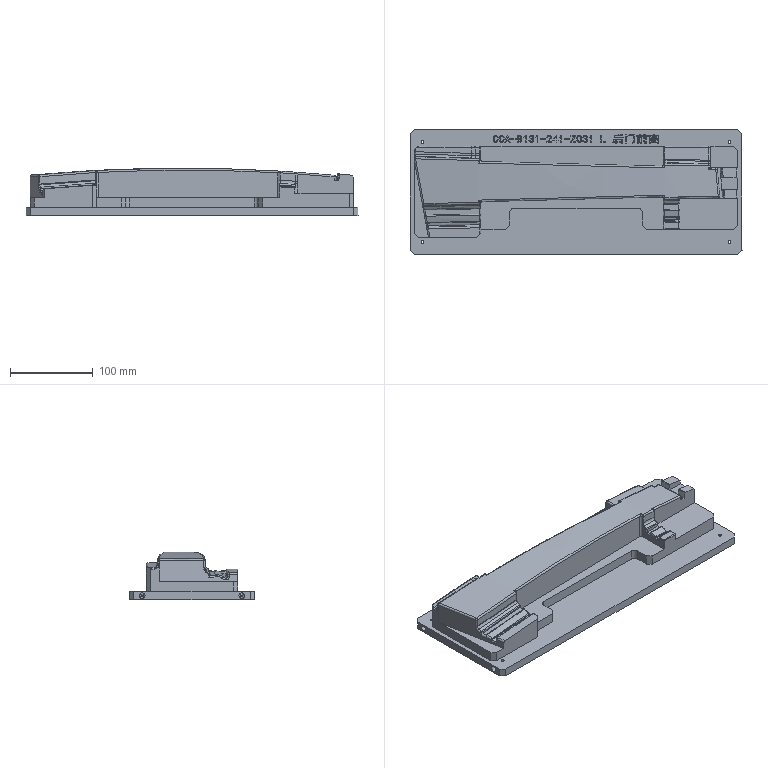NC program | NX | posted with a generic post | part box 400 x 150 x 57.494 mm
Lines 58 to 1056 of 7057:
(A4 , TOOL : D0.5)
N102 M6
N104 G54
N106 G17 G0 G90 X-99.468 Y63.115 S0 M3
N108 G43 Z20.002 H0
N110 Z10.302
N112 G94 G1 X-99.408 Y62.639 Z10.277 F250.
N114 X-99.26 Y62.087 Z10.247
N116 X-99.023 Y61.594 Z10.218
N118 X-98.688 Y61.174 Z10.19
N120 X-98.122 Y60.757 Z10.153
N122 X-98.359 Y60.946 Z10.137
N124 X-98.535 Y61.194 Z10.122
N126 X-98.911 Y61.942 Z10.078
N128 X-99.085 Y62.741 Z10.035
N130 X-99.146 Y63.516 Z9.994
N132 X-99.142 Y64.278 Z9.954
N134 X-99.139 Y64.316 Z9.952
N136 X-99.076 Y65.081
N138 X-98.905 Y65.905
N140 X-98.539 Y66.707
N142 X-98.173 Y67.122
N144 X-98.022 Y67.233
N146 G3 X-99.028 Y66.178 R2.627
N148 X-99.26 Y62.087 R6.192
N150 G1 X-99.023 Y61.594
N152 X-98.688 Y61.174
N154 X-98.268 Y60.845
N156 X-98.122 Y60.757
N158 G2 X-98.535 Y61.194 R2.143
N160 G1 X-98.911 Y61.942
N162 X-99.085 Y62.741
N164 X-99.146 Y63.516
N166 X-99.142 Y64.278
N168 X-99.139 Y64.316
N170 X-98.89 Y64.295
N172 X-98.828 Y65.045
N174 X-98.666 Y65.827
N176 G2 X-95.732 Y67.213 R2.025
N178 G1 X-95.663 Y67.169
N180 X-95.496 Y67.021
N182 X-95.329 Y67.207
N184 X-95.166 Y67.062
N186 X-95.083 Y67.017
N188 X-95.059 Y66.925
N190 X-94.818 Y66.478
N192 X-94.671 Y65.947
N194 X-94.646 Y65.644
N196 X-94.391
N198 X-94.568 Y66.329
N200 X-94.673 Y66.566
N202 X-94.957 Y66.932
N204 G3 X-95.329 Y67.207 R2.627
N206 G1 X-95.496 Y67.021
N208 X-95.333 Y66.875
N210 X-95.279 Y66.807
N212 X-95.051 Y66.384
N214 X-94.918 Y65.903
N216 X-94.876 Y65.394
N218 X-94.13
N220 X-94.222 Y66.097
N222 X-94.335 Y66.421
N224 X-94.456 Y66.696
N226 X-94.773 Y67.103
N228 G3 X-99.254 Y66.284 R2.877
N230 X-99.496 Y61.999 R6.441
N232 G1 X-99.236 Y61.461
N234 X-98.866 Y60.995
N236 X-98.414 Y60.642
N238 G3 X-95.389 Y60.515 R2.952
N240 G1 X-95.508 Y60.735
N242 G3 X-94.923 Y61.161 R2.702
N244 X-94.363 Y62.679 R2.769
N246 G1 X-94.628
N248 X-94.629 Y62.649
N250 X-94.696 Y62.107
N252 X-94.86 Y61.539
N254 X-95.145 Y61.072
N256 X-95.251 Y60.949
N258 X-95.508 Y60.735
N260 X-95.389 Y60.515
N262 G3 X-94.73 Y61.001 R2.952
N264 X-94.087 Y62.929 R3.246
N266 G1 X-94.867
N268 X-94.879 Y62.67
N270 X-94.942 Y62.158
N272 X-95.091 Y61.64
N274 X-95.358 Y61.203
N276 X-95.411 Y61.141
N278 X-95.809 Y60.809
N280 G2 X-98.32 Y61.325 R1.893
N282 G1 X-98.673 Y62.026
N284 X-98.837 Y62.777
N286 X-98.896 Y63.525
N288 X-98.892 Y64.267
N290 X-98.89 Y64.295
N292 X-99.139 Y64.316 Z9.965
N294 Z10.265
N296 G0 Z10.302
N298 X-99.468 Y63.115
N300 Z10.252
N302 G1 X-99.408 Y62.639 Z10.227
N304 X-99.26 Y62.087 Z10.197
N306 X-99.023 Y61.594 Z10.168
N308 X-98.688 Y61.174 Z10.14
N310 X-98.122 Y60.757 Z10.103
N312 X-98.359 Y60.946 Z10.087
N314 X-98.535 Y61.194 Z10.072
N316 X-98.911 Y61.942 Z10.028
N318 X-99.085 Y62.741 Z9.985
N320 X-99.146 Y63.516 Z9.944
N322 X-99.142 Y64.278 Z9.904
N324 X-99.139 Y64.316 Z9.902
N326 X-99.076 Y65.081
N328 X-98.905 Y65.905
N330 X-98.539 Y66.707
N332 X-98.173 Y67.122
N334 X-98.022 Y67.233
N336 G3 X-99.028 Y66.178 R2.627
N338 X-99.26 Y62.087 R6.192
N340 G1 X-99.023 Y61.594
N342 X-98.688 Y61.174
N344 X-98.268 Y60.845
N346 X-98.122 Y60.757
N348 G2 X-98.535 Y61.194 R2.143
N350 G1 X-98.911 Y61.942
N352 X-99.085 Y62.741
N354 X-99.146 Y63.516
N356 X-99.142 Y64.278
N358 X-99.139 Y64.316
N360 X-98.89 Y64.295
N362 X-98.828 Y65.045
N364 X-98.666 Y65.827
N366 G2 X-95.732 Y67.213 R2.025
N368 G1 X-95.663 Y67.169
N370 X-95.496 Y67.021
N372 X-95.329 Y67.207
N374 X-95.166 Y67.062
N376 X-95.083 Y67.017
N378 X-95.059 Y66.925
N380 X-94.818 Y66.478
N382 X-94.671 Y65.947
N384 X-94.646 Y65.644
N386 X-94.391
N388 X-94.568 Y66.329
N390 X-94.673 Y66.566
N392 X-94.957 Y66.932
N394 G3 X-95.329 Y67.207 R2.627
N396 G1 X-95.496 Y67.021
N398 X-95.333 Y66.875
N400 X-95.279 Y66.807
N402 X-95.051 Y66.384
N404 X-94.918 Y65.903
N406 X-94.876 Y65.394
N408 X-94.13
N410 X-94.222 Y66.097
N412 X-94.335 Y66.421
N414 X-94.456 Y66.696
N416 X-94.773 Y67.103
N418 G3 X-99.254 Y66.284 R2.877
N420 X-99.496 Y61.999 R6.441
N422 G1 X-99.236 Y61.461
N424 X-98.866 Y60.995
N426 X-98.414 Y60.642
N428 G3 X-95.389 Y60.515 R2.952
N430 G1 X-95.508 Y60.735
N432 G3 X-94.923 Y61.161 R2.702
N434 X-94.363 Y62.679 R2.769
N436 G1 X-94.628
N438 X-94.629 Y62.649
N440 X-94.696 Y62.107
N442 X-94.86 Y61.539
N444 X-95.145 Y61.072
N446 X-95.251 Y60.949
N448 X-95.508 Y60.735
N450 X-95.389 Y60.515
N452 G3 X-94.73 Y61.001 R2.952
N454 X-94.087 Y62.929 R3.246
N456 G1 X-94.867
N458 X-94.879 Y62.67
N460 X-94.942 Y62.158
N462 X-95.091 Y61.64
N464 X-95.358 Y61.203
N466 X-95.411 Y61.141
N468 X-95.809 Y60.809
N470 G2 X-98.32 Y61.325 R1.893
N472 G1 X-98.673 Y62.026
N474 X-98.837 Y62.777
N476 X-98.896 Y63.525
N478 X-98.892 Y64.267
N480 X-98.89 Y64.295
N482 X-99.139 Y64.316 Z9.915
N484 Z10.215
N486 G0 Z10.252
N488 X-99.468 Y63.115
N490 Z10.202
N492 G1 X-99.408 Y62.639 Z10.177
N494 X-99.26 Y62.087 Z10.147
N496 X-99.023 Y61.594 Z10.118
N498 X-98.688 Y61.174 Z10.09
N500 X-98.122 Y60.757 Z10.053
N502 X-98.359 Y60.946 Z10.037
N504 X-98.535 Y61.194 Z10.022
N506 X-98.911 Y61.942 Z9.978
N508 X-99.085 Y62.741 Z9.935
N510 X-99.146 Y63.516 Z9.894
N512 X-99.142 Y64.278 Z9.854
N514 X-99.139 Y64.316 Z9.852
N516 X-99.076 Y65.081
N518 X-98.905 Y65.905
N520 X-98.539 Y66.707
N522 X-98.173 Y67.122
N524 X-98.022 Y67.233
N526 G3 X-99.028 Y66.178 R2.627
N528 X-99.26 Y62.087 R6.192
N530 G1 X-99.023 Y61.594
N532 X-98.688 Y61.174
N534 X-98.268 Y60.845
N536 X-98.122 Y60.757
N538 G2 X-98.535 Y61.194 R2.143
N540 G1 X-98.911 Y61.942
N542 X-99.085 Y62.741
N544 X-99.146 Y63.516
N546 X-99.142 Y64.278
N548 X-99.139 Y64.316
N550 X-98.89 Y64.295
N552 X-98.828 Y65.045
N554 X-98.666 Y65.827
N556 G2 X-95.732 Y67.213 R2.025
N558 G1 X-95.663 Y67.169
N560 X-95.496 Y67.021
N562 X-95.329 Y67.207
N564 X-95.166 Y67.062
N566 X-95.083 Y67.017
N568 X-95.059 Y66.925
N570 X-94.818 Y66.478
N572 X-94.671 Y65.947
N574 X-94.646 Y65.644
N576 X-94.391
N578 X-94.568 Y66.329
N580 X-94.673 Y66.566
N582 X-94.957 Y66.932
N584 G3 X-95.329 Y67.207 R2.627
N586 G1 X-95.496 Y67.021
N588 X-95.333 Y66.875
N590 X-95.279 Y66.807
N592 X-95.051 Y66.384
N594 X-94.918 Y65.903
N596 X-94.876 Y65.394
N598 X-94.13
N600 X-94.222 Y66.097
N602 X-94.335 Y66.421
N604 X-94.456 Y66.696
N606 X-94.773 Y67.103
N608 G3 X-99.254 Y66.284 R2.877
N610 X-99.496 Y61.999 R6.441
N612 G1 X-99.236 Y61.461
N614 X-98.866 Y60.995
N616 X-98.414 Y60.642
N618 G3 X-95.389 Y60.515 R2.952
N620 G1 X-95.508 Y60.735
N622 G3 X-94.923 Y61.161 R2.702
N624 X-94.363 Y62.679 R2.769
N626 G1 X-94.628
N628 X-94.629 Y62.649
N630 X-94.696 Y62.107
N632 X-94.86 Y61.539
N634 X-95.145 Y61.072
N636 X-95.251 Y60.949
N638 X-95.508 Y60.735
N640 X-95.389 Y60.515
N642 G3 X-94.73 Y61.001 R2.952
N644 X-94.087 Y62.929 R3.246
N646 G1 X-94.867
N648 X-94.879 Y62.67
N650 X-94.942 Y62.158
N652 X-95.091 Y61.64
N654 X-95.358 Y61.203
N656 X-95.411 Y61.141
N658 X-95.809 Y60.809
N660 G2 X-98.32 Y61.325 R1.893
N662 G1 X-98.673 Y62.026
N664 X-98.837 Y62.777
N666 X-98.896 Y63.525
N668 X-98.892 Y64.267
N670 X-98.89 Y64.295
N672 X-99.139 Y64.316 Z9.865
N674 Z10.165
N676 G0 Z10.202
N678 X-99.468 Y63.115
N680 Z10.152
N682 G1 X-99.408 Y62.639 Z10.127
N684 X-99.26 Y62.087 Z10.097
N686 X-99.023 Y61.594 Z10.068
N688 X-98.688 Y61.174 Z10.04
N690 X-98.122 Y60.757 Z10.003
N692 X-98.359 Y60.946 Z9.987
N694 X-98.535 Y61.194 Z9.972
N696 X-98.911 Y61.942 Z9.928
N698 X-99.085 Y62.741 Z9.885
N700 X-99.146 Y63.516 Z9.844
N702 X-99.142 Y64.278 Z9.804
N704 X-99.139 Y64.316 Z9.802
N706 X-99.076 Y65.081
N708 X-98.905 Y65.905
N710 X-98.539 Y66.707
N712 X-98.173 Y67.122
N714 X-98.022 Y67.233
N716 G3 X-99.028 Y66.178 R2.627
N718 X-99.26 Y62.087 R6.192
N720 G1 X-99.023 Y61.594
N722 X-98.688 Y61.174
N724 X-98.268 Y60.845
N726 X-98.122 Y60.757
N728 G2 X-98.535 Y61.194 R2.143
N730 G1 X-98.911 Y61.942
N732 X-99.085 Y62.741
N734 X-99.146 Y63.516
N736 X-99.142 Y64.278
N738 X-99.139 Y64.316
N740 X-98.89 Y64.295
N742 X-98.828 Y65.045
N744 X-98.666 Y65.827
N746 G2 X-95.732 Y67.213 R2.025
N748 G1 X-95.663 Y67.169
N750 X-95.496 Y67.021
N752 X-95.329 Y67.207
N754 X-95.166 Y67.062
N756 X-95.083 Y67.017
N758 X-95.059 Y66.925
N760 X-94.818 Y66.478
N762 X-94.671 Y65.947
N764 X-94.646 Y65.644
N766 X-94.391
N768 X-94.568 Y66.329
N770 X-94.673 Y66.566
N772 X-94.957 Y66.932
N774 G3 X-95.329 Y67.207 R2.627
N776 G1 X-95.496 Y67.021
N778 X-95.333 Y66.875
N780 X-95.279 Y66.807
N782 X-95.051 Y66.384
N784 X-94.918 Y65.903
N786 X-94.876 Y65.394
N788 X-94.13
N790 X-94.222 Y66.097
N792 X-94.335 Y66.421
N794 X-94.456 Y66.696
N796 X-94.773 Y67.103
N798 G3 X-99.254 Y66.284 R2.877
N800 X-99.496 Y61.999 R6.441
N802 G1 X-99.236 Y61.461
N804 X-98.866 Y60.995
N806 X-98.414 Y60.642
N808 G3 X-95.389 Y60.515 R2.952
N810 G1 X-95.508 Y60.735
N812 G3 X-94.923 Y61.161 R2.702
N814 X-94.363 Y62.679 R2.769
N816 G1 X-94.628
N818 X-94.629 Y62.649
N820 X-94.696 Y62.107
N822 X-94.86 Y61.539
N824 X-95.145 Y61.072
N826 X-95.251 Y60.949
N828 X-95.508 Y60.735
N830 X-95.389 Y60.515
N832 G3 X-94.73 Y61.001 R2.952
N834 X-94.087 Y62.929 R3.246
N836 G1 X-94.867
N838 X-94.879 Y62.67
N840 X-94.942 Y62.158
N842 X-95.091 Y61.64
N844 X-95.358 Y61.203
N846 X-95.411 Y61.141
N848 X-95.809 Y60.809
N850 G2 X-98.32 Y61.325 R1.893
N852 G1 X-98.673 Y62.026
N854 X-98.837 Y62.777
N856 X-98.896 Y63.525
N858 X-98.892 Y64.267
N860 X-98.89 Y64.295
N862 X-99.139 Y64.316 Z9.815
N864 Z10.115
N866 G0 Z20.002
N868 X-92.265 Y63.117
N870 Z10.302
N872 G1 X-92.12 Y62.315 Z10.259
N874 X-91.994 Y61.952 Z10.239
N876 X-91.821 Y61.594 Z10.218
N878 X-91.487 Y61.174 Z10.19
N880 X-90.921 Y60.757 Z10.153
N882 X-91.158 Y60.946 Z10.137
N884 X-91.333 Y61.194 Z10.122
N886 X-91.71 Y61.942 Z10.078
N888 X-91.884 Y62.741 Z10.035
N890 X-91.945 Y63.516 Z9.994
N892 X-91.941 Y64.278 Z9.954
N894 X-91.938 Y64.316 Z9.952
N896 X-91.875 Y65.081
N898 X-91.704 Y65.905
N900 X-91.337 Y66.707
N902 X-90.972 Y67.122
N904 X-90.821 Y67.233
N906 G3 X-91.826 Y66.178 R2.627
N908 X-91.994 Y61.952 R6.118
N910 G1 X-91.821 Y61.594
N912 X-91.487 Y61.174
N914 X-91.067 Y60.845
N916 X-90.921 Y60.757
N918 G2 X-91.333 Y61.194 R2.143
N920 G1 X-91.71 Y61.942
N922 X-91.884 Y62.741
N924 X-91.945 Y63.516
N926 X-91.941 Y64.278
N928 X-91.938 Y64.316
N930 X-91.689 Y64.295
N932 X-91.627 Y65.045
N934 X-91.465 Y65.827
N936 G2 X-88.53 Y67.213 R2.025
N938 G1 X-88.461 Y67.169
N940 X-88.295 Y67.021
N942 X-88.128 Y67.207
N944 X-87.965 Y67.062
N946 X-87.882 Y67.017
N948 X-87.857 Y66.925
N950 X-87.617 Y66.478
N952 X-87.47 Y65.947
N954 X-87.445 Y65.644
N956 X-87.191
N958 X-87.303 Y66.185
N960 X-87.46 Y66.541
N962 X-87.476 Y66.572
N964 X-87.755 Y66.932
N966 G3 X-88.128 Y67.207 R2.627
N968 G1 X-88.295 Y67.021
N970 X-88.131 Y66.875
N972 X-88.078 Y66.807
N974 X-87.85 Y66.384
N976 X-87.717 Y65.903
N978 X-87.675 Y65.394
N980 X-86.93
N982 G3 X-87.572 Y67.103 R2.398
N984 X-92.053 Y66.284 R2.877
N986 X-92.226 Y61.857 R6.364
N988 G1 X-92.034 Y61.461
N990 X-91.664 Y60.995
N992 X-91.213 Y60.642
N994 G3 X-88.187 Y60.515 R2.952
N996 G1 X-88.306 Y60.735
N998 G3 X-87.732 Y61.151 R2.702
N1000 X-87.155 Y62.679 R2.877
N1002 G1 X-87.427
N1004 X-87.428 Y62.649
N1006 X-87.495 Y62.107
N1008 X-87.659 Y61.539
N1010 X-87.943 Y61.072
N1012 X-88.05 Y60.949
N1014 X-88.306 Y60.735
N1016 X-88.187 Y60.515
N1018 G3 X-87.545 Y60.984 R2.952
N1020 G1 X-87.196 Y61.535
N1022 X-87.044 Y61.946
N1024 X-87.017 Y62.033
N1026 X-86.883 Y62.929
N1028 X-87.666
N1030 X-87.677 Y62.67
N1032 X-87.741 Y62.158
N1034 X-87.89 Y61.64
N1036 X-88.157 Y61.203
N1038 X-88.21 Y61.141
N1040 X-88.608 Y60.809
N1042 G2 X-91.119 Y61.325 R1.893
N1044 G1 X-91.472 Y62.026
N1046 X-91.636 Y62.777
N1048 X-91.695 Y63.525
N1050 X-91.691 Y64.267
N1052 X-91.689 Y64.295
N1054 X-91.938 Y64.316 Z9.965
N1056 Z10.265
N1058 G0 Z10.302
N1060 X-92.265 Y63.117
N1062 Z10.252
N1064 G1 X-92.12 Y62.315 Z10.209
N1066 X-91.994 Y61.952 Z10.189
N1068 X-91.821 Y61.594 Z10.168
N1070 X-91.487 Y61.174 Z10.14
N1072 X-90.921 Y60.757 Z10.103
N1074 X-91.158 Y60.946 Z10.087
N1076 X-91.333 Y61.194 Z10.072
N1078 X-91.71 Y61.942 Z10.028
N1080 X-91.884 Y62.741 Z9.985
N1082 X-91.945 Y63.516 Z9.944
N1084 X-91.941 Y64.278 Z9.904
N1086 X-91.938 Y64.316 Z9.902
N1088 X-91.875 Y65.081
N1090 X-91.704 Y65.905
N1092 X-91.337 Y66.707
N1094 X-90.972 Y67.122
N1096 X-90.821 Y67.233
N1098 G3 X-91.826 Y66.178 R2.627
N1100 X-91.994 Y61.952 R6.118
N1102 G1 X-91.821 Y61.594
N1104 X-91.487 Y61.174
N1106 X-91.067 Y60.845
N1108 X-90.921 Y60.757
N1110 G2 X-91.333 Y61.194 R2.143
N1112 G1 X-91.71 Y61.942
N1114 X-91.884 Y62.741
N1116 X-91.945 Y63.516
N1118 X-91.941 Y64.278
N1120 X-91.938 Y64.316
N1122 X-91.689 Y64.295
N1124 X-91.627 Y65.045
N1126 X-91.465 Y65.827
N1128 G2 X-88.53 Y67.213 R2.025
N1130 G1 X-88.461 Y67.169
N1132 X-88.295 Y67.021
N1134 X-88.128 Y67.207
N1136 X-87.965 Y67.062
N1138 X-87.882 Y67.017
N1140 X-87.857 Y66.925
N1142 X-87.617 Y66.478
N1144 X-87.47 Y65.947
N1146 X-87.445 Y65.644
N1148 X-87.191
N1150 X-87.303 Y66.185
N1152 X-87.46 Y66.541
N1154 X-87.476 Y66.572
N1156 X-87.755 Y66.932
N1158 G3 X-88.128 Y67.207 R2.627
N1160 G1 X-88.295 Y67.021
N1162 X-88.131 Y66.875
N1164 X-88.078 Y66.807
N1166 X-87.85 Y66.384
N1168 X-87.717 Y65.903
N1170 X-87.675 Y65.394
N1172 X-86.93
N1174 G3 X-87.572 Y67.103 R2.398
N1176 X-92.053 Y66.284 R2.877
N1178 X-92.226 Y61.857 R6.364
N1180 G1 X-92.034 Y61.461
N1182 X-91.664 Y60.995
N1184 X-91.213 Y60.642
N1186 G3 X-88.187 Y60.515 R2.952
N1188 G1 X-88.306 Y60.735
N1190 G3 X-87.732 Y61.151 R2.702
N1192 X-87.155 Y62.679 R2.877
N1194 G1 X-87.427
N1196 X-87.428 Y62.649
N1198 X-87.495 Y62.107
N1200 X-87.659 Y61.539
N1202 X-87.943 Y61.072
N1204 X-88.05 Y60.949
N1206 X-88.306 Y60.735
N1208 X-88.187 Y60.515
N1210 G3 X-87.545 Y60.984 R2.952
N1212 G1 X-87.196 Y61.535
N1214 X-87.044 Y61.946
N1216 X-87.017 Y62.033
N1218 X-86.883 Y62.929
N1220 X-87.666
N1222 X-87.677 Y62.67
N1224 X-87.741 Y62.158
N1226 X-87.89 Y61.64
N1228 X-88.157 Y61.203
N1230 X-88.21 Y61.141
N1232 X-88.608 Y60.809
N1234 G2 X-91.119 Y61.325 R1.893
N1236 G1 X-91.472 Y62.026
N1238 X-91.636 Y62.777
N1240 X-91.695 Y63.525
N1242 X-91.691 Y64.267
N1244 X-91.689 Y64.295
N1246 X-91.938 Y64.316 Z9.915
N1248 Z10.215
N1250 G0 Z10.252
N1252 X-92.265 Y63.117
N1254 Z10.202
N1256 G1 X-92.12 Y62.315 Z10.159
N1258 X-91.994 Y61.952 Z10.139
N1260 X-91.821 Y61.594 Z10.118
N1262 X-91.487 Y61.174 Z10.09
N1264 X-90.921 Y60.757 Z10.053
N1266 X-91.158 Y60.946 Z10.037
N1268 X-91.333 Y61.194 Z10.022
N1270 X-91.71 Y61.942 Z9.978
N1272 X-91.884 Y62.741 Z9.935
N1274 X-91.945 Y63.516 Z9.894
N1276 X-91.941 Y64.278 Z9.854
N1278 X-91.938 Y64.316 Z9.852
N1280 X-91.875 Y65.081
N1282 X-91.704 Y65.905
N1284 X-91.337 Y66.707
N1286 X-90.972 Y67.122
N1288 X-90.821 Y67.233
N1290 G3 X-91.826 Y66.178 R2.627
N1292 X-91.994 Y61.952 R6.118
N1294 G1 X-91.821 Y61.594
N1296 X-91.487 Y61.174
N1298 X-91.067 Y60.845
N1300 X-90.921 Y60.757
N1302 G2 X-91.333 Y61.194 R2.143
N1304 G1 X-91.71 Y61.942
N1306 X-91.884 Y62.741
N1308 X-91.945 Y63.516
N1310 X-91.941 Y64.278
N1312 X-91.938 Y64.316
N1314 X-91.689 Y64.295
N1316 X-91.627 Y65.045
N1318 X-91.465 Y65.827
N1320 G2 X-88.53 Y67.213 R2.025
N1322 G1 X-88.461 Y67.169
N1324 X-88.295 Y67.021
N1326 X-88.128 Y67.207
N1328 X-87.965 Y67.062
N1330 X-87.882 Y67.017
N1332 X-87.857 Y66.925
N1334 X-87.617 Y66.478
N1336 X-87.47 Y65.947
N1338 X-87.445 Y65.644
N1340 X-87.191
N1342 X-87.303 Y66.185
N1344 X-87.46 Y66.541
N1346 X-87.476 Y66.572
N1348 X-87.755 Y66.932
N1350 G3 X-88.128 Y67.207 R2.627
N1352 G1 X-88.295 Y67.021
N1354 X-88.131 Y66.875
N1356 X-88.078 Y66.807
N1358 X-87.85 Y66.384
N1360 X-87.717 Y65.903
N1362 X-87.675 Y65.394
N1364 X-86.93
N1366 G3 X-87.572 Y67.103 R2.398
N1368 X-92.053 Y66.284 R2.877
N1370 X-92.226 Y61.857 R6.364
N1372 G1 X-92.034 Y61.461
N1374 X-91.664 Y60.995
N1376 X-91.213 Y60.642
N1378 G3 X-88.187 Y60.515 R2.952
N1380 G1 X-88.306 Y60.735
N1382 G3 X-87.732 Y61.151 R2.702
N1384 X-87.155 Y62.679 R2.877
N1386 G1 X-87.427
N1388 X-87.428 Y62.649
N1390 X-87.495 Y62.107
N1392 X-87.659 Y61.539
N1394 X-87.943 Y61.072
N1396 X-88.05 Y60.949
N1398 X-88.306 Y60.735
N1400 X-88.187 Y60.515
N1402 G3 X-87.545 Y60.984 R2.952
N1404 G1 X-87.196 Y61.535
N1406 X-87.044 Y61.946
N1408 X-87.017 Y62.033
N1410 X-86.883 Y62.929
N1412 X-87.666
N1414 X-87.677 Y62.67
N1416 X-87.741 Y62.158
N1418 X-87.89 Y61.64
N1420 X-88.157 Y61.203
N1422 X-88.21 Y61.141
N1424 X-88.608 Y60.809
N1426 G2 X-91.119 Y61.325 R1.893
N1428 G1 X-91.472 Y62.026
N1430 X-91.636 Y62.777
N1432 X-91.695 Y63.525
N1434 X-91.691 Y64.267
N1436 X-91.689 Y64.295
N1438 X-91.938 Y64.316 Z9.865
N1440 Z10.165
N1442 G0 Z10.202
N1444 X-92.265 Y63.117
N1446 Z10.152
N1448 G1 X-92.12 Y62.315 Z10.109
N1450 X-91.994 Y61.952 Z10.089
N1452 X-91.821 Y61.594 Z10.068
N1454 X-91.487 Y61.174 Z10.04
N1456 X-90.921 Y60.757 Z10.003
N1458 X-91.158 Y60.946 Z9.987
N1460 X-91.333 Y61.194 Z9.972
N1462 X-91.71 Y61.942 Z9.928
N1464 X-91.884 Y62.741 Z9.885
N1466 X-91.945 Y63.516 Z9.844
N1468 X-91.941 Y64.278 Z9.804
N1470 X-91.938 Y64.316 Z9.802
N1472 X-91.875 Y65.081
N1474 X-91.704 Y65.905
N1476 X-91.337 Y66.707
N1478 X-90.972 Y67.122
N1480 X-90.821 Y67.233
N1482 G3 X-91.826 Y66.178 R2.627
N1484 X-91.994 Y61.952 R6.118
N1486 G1 X-91.821 Y61.594
N1488 X-91.487 Y61.174
N1490 X-91.067 Y60.845
N1492 X-90.921 Y60.757
N1494 G2 X-91.333 Y61.194 R2.143
N1496 G1 X-91.71 Y61.942
N1498 X-91.884 Y62.741
N1500 X-91.945 Y63.516
N1502 X-91.941 Y64.278
N1504 X-91.938 Y64.316
N1506 X-91.689 Y64.295
N1508 X-91.627 Y65.045
N1510 X-91.465 Y65.827
N1512 G2 X-88.53 Y67.213 R2.025
N1514 G1 X-88.461 Y67.169
N1516 X-88.295 Y67.021
N1518 X-88.128 Y67.207
N1520 X-87.965 Y67.062
N1522 X-87.882 Y67.017
N1524 X-87.857 Y66.925
N1526 X-87.617 Y66.478
N1528 X-87.47 Y65.947
N1530 X-87.445 Y65.644
N1532 X-87.191
N1534 X-87.303 Y66.185
N1536 X-87.46 Y66.541
N1538 X-87.476 Y66.572
N1540 X-87.755 Y66.932
N1542 G3 X-88.128 Y67.207 R2.627
N1544 G1 X-88.295 Y67.021
N1546 X-88.131 Y66.875
N1548 X-88.078 Y66.807
N1550 X-87.85 Y66.384
N1552 X-87.717 Y65.903
N1554 X-87.675 Y65.394
N1556 X-86.93
N1558 G3 X-87.572 Y67.103 R2.398
N1560 X-92.053 Y66.284 R2.877
N1562 X-92.226 Y61.857 R6.364
N1564 G1 X-92.034 Y61.461
N1566 X-91.664 Y60.995
N1568 X-91.213 Y60.642
N1570 G3 X-88.187 Y60.515 R2.952
N1572 G1 X-88.306 Y60.735
N1574 G3 X-87.732 Y61.151 R2.702
N1576 X-87.155 Y62.679 R2.877
N1578 G1 X-87.427
N1580 X-87.428 Y62.649
N1582 X-87.495 Y62.107
N1584 X-87.659 Y61.539
N1586 X-87.943 Y61.072
N1588 X-88.05 Y60.949
N1590 X-88.306 Y60.735
N1592 X-88.187 Y60.515
N1594 G3 X-87.545 Y60.984 R2.952
N1596 G1 X-87.196 Y61.535
N1598 X-87.044 Y61.946
N1600 X-87.017 Y62.033
N1602 X-86.883 Y62.929
N1604 X-87.666
N1606 X-87.677 Y62.67
N1608 X-87.741 Y62.158
N1610 X-87.89 Y61.64
N1612 X-88.157 Y61.203
N1614 X-88.21 Y61.141
N1616 X-88.608 Y60.809
N1618 G2 X-91.119 Y61.325 R1.893
N1620 G1 X-91.472 Y62.026
N1622 X-91.636 Y62.777
N1624 X-91.695 Y63.525
N1626 X-91.691 Y64.267
N1628 X-91.689 Y64.295
N1630 X-91.938 Y64.316 Z9.815
N1632 Z10.115
N1634 G0 Z20.002
N1636 X-82.06 Y65.643
N1638 Z10.302
N1640 G1 X-81.364 Y63.443 Z10.181
N1642 X-81.328 Y63.327 Z10.175
N1644 X-81.396 Y63.227 Z10.169
N1646 X-81.088 Y63.189 Z10.152
N1648 X-82.34 Y66.791 Z9.952
N1650 X-82.553 Y66.717
N1652 X-82.56 Y66.738
N1654 X-82.575 Y66.696
N1656 X-82.545
N1658 X-82.553 Y66.717
N1660 X-82.34 Y66.791
N1662 X-82.532 Y67.342
N1664 X-82.588
N1666 X-84.032 Y63.189
N1668 G2 X-83.797 Y63.227 R0.75
N1670 G1 X-83.724
N1672 G2 X-83.755 Y63.443 R0.25
N1674 G1 X-82.854 Y66.296
N1676 G2 X-82.615 Y66.471 R0.25
N1678 G1 X-82.504
N1680 G2 X-82.266 Y66.296 R0.25
N1682 G1 X-81.364 Y63.443
N1684 G2 X-81.396 Y63.227 R0.25
N1686 G1 X-81.323
N1688 G2 X-81.088 Y63.189 R0.75
N1690 G1 X-82.34 Y66.791
N1692 X-82.104 Y66.873
N1694 X-82.354 Y67.592
N1696 X-82.766
N1698 X-85.232 Y60.498
N1700 X-84.951
N1702 X-84.273 Y62.628
N1704 G2 X-83.797 Y62.977 R0.5
N1706 G1 X-81.323
N1708 G2 X-80.847 Y62.628 R0.5
N1710 G1 X-80.169 Y60.498
N1712 X-79.888
N1714 X-82.104 Y66.873
N1716 X-81.868 Y66.955
N1718 X-82.176 Y67.842
N1720 X-82.944
N1722 X-85.583 Y60.248
N1724 X-84.768
N1726 X-84.035 Y62.552
N1728 G2 X-83.797 Y62.727 R0.25
N1730 G1 X-81.323
N1732 G2 X-81.085 Y62.552 R0.25
N1734 G1 X-80.352 Y60.248
N1736 X-79.536
N1738 X-81.868 Y66.955
N1740 X-82.104 Y66.873 Z9.965
N1742 Z10.265
N1744 G0 Z10.302
N1746 X-82.06 Y65.643
N1748 Z10.252
N1750 G1 X-81.364 Y63.443 Z10.131
N1752 X-81.328 Y63.327 Z10.125
N1754 X-81.396 Y63.227 Z10.119
N1756 X-81.088 Y63.189 Z10.102
N1758 X-82.34 Y66.791 Z9.902
N1760 X-82.553 Y66.717
N1762 X-82.56 Y66.738
N1764 X-82.575 Y66.696
N1766 X-82.545
N1768 X-82.553 Y66.717
N1770 X-82.34 Y66.791
N1772 X-82.532 Y67.342
N1774 X-82.588
N1776 X-84.032 Y63.189
N1778 G2 X-83.797 Y63.227 R0.75
N1780 G1 X-83.724
N1782 G2 X-83.755 Y63.443 R0.25
N1784 G1 X-82.854 Y66.296
N1786 G2 X-82.615 Y66.471 R0.25
N1788 G1 X-82.504
N1790 G2 X-82.266 Y66.296 R0.25
N1792 G1 X-81.364 Y63.443
N1794 G2 X-81.396 Y63.227 R0.25
N1796 G1 X-81.323
N1798 G2 X-81.088 Y63.189 R0.75
N1800 G1 X-82.34 Y66.791
N1802 X-82.104 Y66.873
N1804 X-82.354 Y67.592
N1806 X-82.766
N1808 X-85.232 Y60.498
N1810 X-84.951
N1812 X-84.273 Y62.628
N1814 G2 X-83.797 Y62.977 R0.5
N1816 G1 X-81.323
N1818 G2 X-80.847 Y62.628 R0.5
N1820 G1 X-80.169 Y60.498
N1822 X-79.888
N1824 X-82.104 Y66.873
N1826 X-81.868 Y66.955
N1828 X-82.176 Y67.842
N1830 X-82.944
N1832 X-85.583 Y60.248
N1834 X-84.768
N1836 X-84.035 Y62.552
N1838 G2 X-83.797 Y62.727 R0.25
N1840 G1 X-81.323
N1842 G2 X-81.085 Y62.552 R0.25
N1844 G1 X-80.352 Y60.248
N1846 X-79.536
N1848 X-81.868 Y66.955
N1850 X-82.104 Y66.873 Z9.915
N1852 Z10.215
N1854 G0 Z10.252
N1856 X-82.06 Y65.643
N1858 Z10.202
N1860 G1 X-81.364 Y63.443 Z10.081
N1862 X-81.328 Y63.327 Z10.075
N1864 X-81.396 Y63.227 Z10.069
N1866 X-81.088 Y63.189 Z10.052
N1868 X-82.34 Y66.791 Z9.852
N1870 X-82.553 Y66.717
N1872 X-82.56 Y66.738
N1874 X-82.575 Y66.696
N1876 X-82.545
N1878 X-82.553 Y66.717
N1880 X-82.34 Y66.791
N1882 X-82.532 Y67.342
N1884 X-82.588
N1886 X-84.032 Y63.189
N1888 G2 X-83.797 Y63.227 R0.75
N1890 G1 X-83.724
N1892 G2 X-83.755 Y63.443 R0.25
N1894 G1 X-82.854 Y66.296
N1896 G2 X-82.615 Y66.471 R0.25
N1898 G1 X-82.504
N1900 G2 X-82.266 Y66.296 R0.25
N1902 G1 X-81.364 Y63.443
N1904 G2 X-81.396 Y63.227 R0.25
N1906 G1 X-81.323
N1908 G2 X-81.088 Y63.189 R0.75
N1910 G1 X-82.34 Y66.791
N1912 X-82.104 Y66.873
N1914 X-82.354 Y67.592
N1916 X-82.766
N1918 X-85.232 Y60.498
N1920 X-84.951
N1922 X-84.273 Y62.628
N1924 G2 X-83.797 Y62.977 R0.5
N1926 G1 X-81.323
N1928 G2 X-80.847 Y62.628 R0.5
N1930 G1 X-80.169 Y60.498
N1932 X-79.888
N1934 X-82.104 Y66.873
N1936 X-81.868 Y66.955
N1938 X-82.176 Y67.842
N1940 X-82.944
N1942 X-85.583 Y60.248
N1944 X-84.768
N1946 X-84.035 Y62.552
N1948 G2 X-83.797 Y62.727 R0.25
N1950 G1 X-81.323
N1952 G2 X-81.085 Y62.552 R0.25
N1954 G1 X-80.352 Y60.248
N1956 X-79.536
N1958 X-81.868 Y66.955
N1960 X-82.104 Y66.873 Z9.865
N1962 Z10.165
N1964 G0 Z10.202
N1966 X-82.06 Y65.643
N1968 Z10.152
N1970 G1 X-81.364 Y63.443 Z10.031
N1972 X-81.328 Y63.327 Z10.025
N1974 X-81.396 Y63.227 Z10.019
N1976 X-81.088 Y63.189 Z10.002
N1978 X-82.34 Y66.791 Z9.802
N1980 X-82.553 Y66.717
N1982 X-82.56 Y66.738
N1984 X-82.575 Y66.696
N1986 X-82.545
N1988 X-82.553 Y66.717
N1990 X-82.34 Y66.791
N1992 X-82.532 Y67.342
N1994 X-82.588
N1996 X-84.032 Y63.189
N1998 G2 X-83.797 Y63.227 R0.75
N2000 G1 X-83.724
N2002 G2 X-83.755 Y63.443 R0.25
N2004 G1 X-82.854 Y66.296
N2006 G2 X-82.615 Y66.471 R0.25
N2008 G1 X-82.504
N2010 G2 X-82.266 Y66.296 R0.25
N2012 G1 X-81.364 Y63.443
N2014 G2 X-81.396 Y63.227 R0.25
N2016 G1 X-81.323
N2018 G2 X-81.088 Y63.189 R0.75
N2020 G1 X-82.34 Y66.791
N2022 X-82.104 Y66.873
N2024 X-82.354 Y67.592
N2026 X-82.766
N2028 X-85.232 Y60.498
N2030 X-84.951
N2032 X-84.273 Y62.628
N2034 G2 X-83.797 Y62.977 R0.5
N2036 G1 X-81.323
N2038 G2 X-80.847 Y62.628 R0.5
N2040 G1 X-80.169 Y60.498
N2042 X-79.888
N2044 X-82.104 Y66.873
N2046 X-81.868 Y66.955
N2048 X-82.176 Y67.842
N2050 X-82.944
N2052 X-85.583 Y60.248
N2054 X-84.768
N2056 X-84.035 Y62.552
N2058 G2 X-83.797 Y62.727 R0.25
N2060 G1 X-81.323
N2062 G2 X-81.085 Y62.552 R0.25
N2064 G1 X-80.352 Y60.248
N2066 X-79.536
N2068 X-81.868 Y66.955
N2070 X-82.104 Y66.873 Z9.815
N2072 Z10.115
N2074 G0 Z20.002
N2076 X-75.932 Y63.99
N2078 Z10.302
N2080 G1 X-72.458 Z10.12
N2082 Y64.238 Z10.107
N2084 X-75.414 Z9.952
N2086 X-78.37
N2088 Y63.99
N2090 X-72.458
N2092 Y64.238